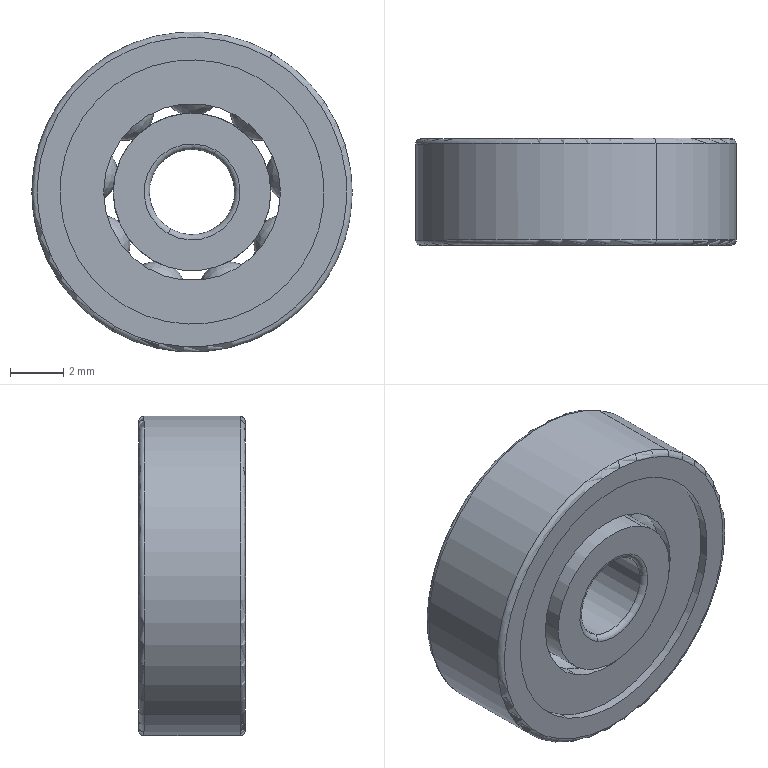Part | SolidWorks | features BaseBody 1 | 1 solid | 160 faces | box 12.003 x 4.011 x 12 mm | volume 319.193 mm3 | sphere 72 | torus 38 | plane 26 | cylinder 24 | commonest cylinder face diameters 9.9 x8 5.9 x4 6.626 x4 3.2 x2 7.295 x2 8.505 x2